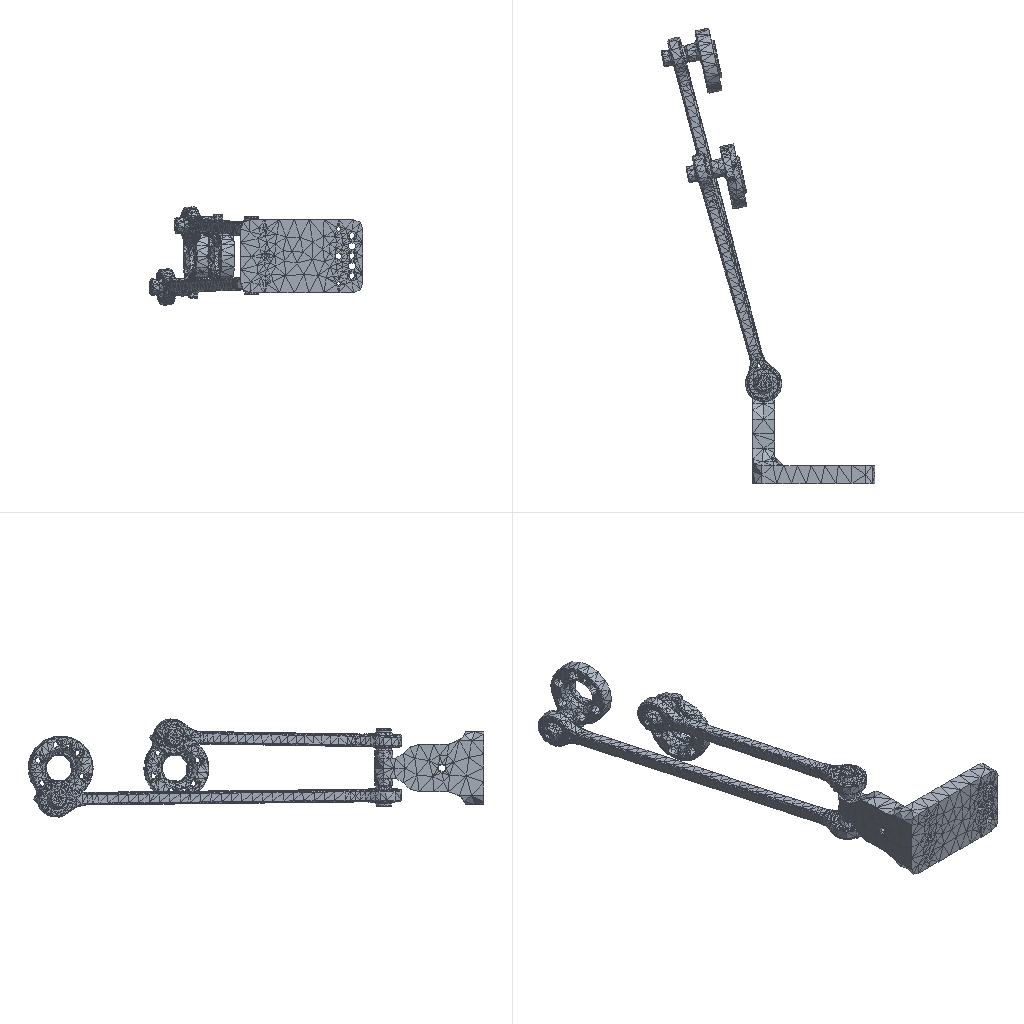Simulation study | ansys workbench
Set-up summary:
category,name,step,type,value,unit,region
solver,ansys_workbench
units,mm-N-s-tonne (MPa),,stated,"/units,MPA"
analysis,LS1,,static
load_step,LS1,LS1,static,nsubst=1; time=1
mesh,nodes,,,43190
mesh,elements,,,31135
element_type,SOLID187,,,21607
element_type,CONTA174,,,5036
element_type,TARGE170,,,4234
element_type,SURF154,,,258
material,Structural Steel,,E,200000,tonne s^-2 mm^-1
material,Structural Steel,,nu,0.3
material,Structural Steel,,density,7.85e-09,tonne mm^-3
material,Structural Steel,,conductivity,60.5,tonne mm s^-3 C^-1
material,Structural Steel,,specific_heat,4.34e+08,mm^2 s^-2 C^-1
material,Structural Steel,,cte,1.2e-05,C^-1
material,Structural Steel,,permeability,10000
material,Structural Steel,,resistivity,0.00017,ohm mm
load,Define Force Using Surface Effect Elements,LS1,surface-effect pres face 2,0.1,,SURF154 #100
bc,Fixed Supports,model,fixed,[dofs=ALL],,_FIXEDSU
bc,,LS1,fixed,"[dofs=ROTX,ROTY,ROTZ,UX,UZ n=5]",,node list
contact,1,,bonded (always),element=CONTA174
contact,Contact Region 2,,bonded (always),element=CONTA174
contact,Contact Region 3,,bonded (always),element=CONTA174
contact,Contact Region 5,,bonded (always),element=CONTA174
contact,Contact Region 6,,bonded (always),element=CONTA174
contact,Contact Region 8,,bonded (always),element=CONTA174
contact,Contact Region 9,,bonded (always),element=CONTA174
contact,Contact Region 10,,bonded (always),element=CONTA174
contact,Contact Region 11,,bonded (always),element=CONTA174
contact,Contact Region 12,,bonded (always),element=CONTA174
contact,Contact Region 13,,bonded (always),element=CONTA174
contact,Contact Region 15,,bonded (always),element=CONTA174
contact,Contact Region 17,,bonded (always),element=CONTA174
contact,Contact Region 18,,bonded (always),element=CONTA174
contact,Contact Region 19,,bonded (always),element=CONTA174
contact,Contact Region 21,,bonded (always),element=CONTA174
contact,Contact Region 23,,bonded (always),element=CONTA174
contact,Contact Region 24,,bonded (always),element=CONTA174
contact,Contact Region 25,,bonded (always),element=CONTA174
contact,? - ? To ?,,bonded (always),element=CONTA174
contact,? - ? To ?,,bonded (always),element=CONTA174
contact,Contact Region 22,,bonded (always),element=CONTA174
contact,Contact Region 26,,bonded (always),element=CONTA174
contact,Contact Region 27,,bonded (always),element=CONTA174
contact,Contact Region 28,,bonded (always),element=CONTA174
contact,Contact Region 29,,bonded (always),element=CONTA174
contact,Contact Region 30,,bonded (always),element=CONTA174
contact,? - ? To ?,,bonded (always),element=CONTA174
contact,? - ? To ?,,bonded (always),element=CONTA174
contact,contact 30,,bonded (always),element=CONTA174
contact,contact 31,,bonded (always),element=CONTA174
contact,contact 32,,bonded (always),element=CONTA174
contact,contact 33,,bonded (always),element=CONTA174
contact,contact 34,,bonded (always),element=CONTA174
contact,contact 35,,bonded (always),element=CONTA174
contact,contact 36,,bonded (always),element=CONTA174
contact,contact 37,,bonded (always),element=CONTA174
contact,contact 38,,bonded (always),element=CONTA174
named_set,_FIXEDSU,,node,746
named_set,REMOTEDISPALL,,node,1
Ansys APDL input file, long lists of numbers shortened:
/batch
/config,noeldb,1     ! force off writing results to database
*get,_wallstrt,active,,time,wall
! ANSYS input file written by Workbench version 2024 R2
! File used for geometry attach:
/title,wbnew--____ (A5)
! ****** Begin Custom Load Command Snippet ******
/COM, ACT Extensions:
/COM,     LSDYNA, 2024.2
/COM,/COM,     ANSYSMotion, 2024.2
/COM,
! ****** End   Custom Load Command Snippet ******
*DIM,_wb_ProjectScratch_dir,string,248
_wb_ProjectScratch_dir(1) = ''
*DIM,_wb_SolverFiles_dir,string,248
_wb_SolverFiles_dir(1) = ''
*DIM,_wb_userfiles_dir,string,248
_wb_userfiles_dir(1) = ''
/com,--- Data in consistent NMM units. See Solving Units in the help system for more information.
/units,MPA
/nopr
/wb,file,start              !  signify a WB generated input file
/prep7
! Turn off shape checking because checks already performed inside WB mesher.
! See help system for more information.
SHPP,OFF,,NOWARN
/nolist
etcon,set             ! allow ANSYS to choose best KEYOP's for 180x elements, resets any applicable keyopt to MAPDL defaults
/com,*********** Nodes for the whole assembly ***********
nblock,3,,47499
(1i9,3e20.9e3)
        1    -2.462083880E+01     5.415586931E+01     1.953544541E+01
! (43180 more lines like these left out)
-1
/com,*********** Nodes for all Remote Points ***********
nblock,3
(1i9,3e20.9e3)
    43192    -1.163425513E+00    -1.361181627E-06     3.324158420E-02
! (8 more lines like these left out)
-1
/wb,elem,start            !  set before creation of elements
/com,*********** Elements for Body 1 'BNN51-GEG6C_ASM|BNN51-GEG6C-1|BNN51-GEG6C-1' ***********
et,1,187
eblock,19,solid,,195
(19i9)
        1        1        1        1        0        0        0        0       10        0        1       27       76       84       77      250      436      252      251
! (389 more lines like these left out)
-1
/com,*********** Elements for Body 2 'BNN51-GEG6C_ASM|BNN51-GEG6C-2|BNN51-GEG6C-2' ***********
et,2,187
eblock,19,solid,,134
(19i9)
        2        2        2        2        0        0        0        0       10        0      196      455      508      507      495      609      787      608      607
! (267 more lines like these left out)
-1
/com,*********** Elements for Body 3 'BNN51-GEG6C5097213_ASM|BNN51-GEG6C-2|BNN51-GEG6C-2' ***********
et,3,187
eblock,19,solid,,134
(19i9)
        3        3        3        3        0        0        0        0       10        0      330      805      858      857      845      959     1137      958      957
! (267 more lines like these left out)
-1
/com,*********** Elements for Body 4 'BNN51-GEG6C5097213_ASM|BNN51-GEG6C-1|BNN51-GEG6C-1' ***********
et,4,187
eblock,19,solid,,195
(19i9)
        4        4        4        4        0        0        0        0       10        0      464     1172     1221     1229     1222     1395     1581     1397     1396
! (389 more lines like these left out)
-1
/com,*********** Elements for Body 5 'GHA-0000182_ASM|BNN51-GEG6C6483096_ASM|BNN51-GEG6C-1|BNN51-GEG6C-1' ***********
et,5,187
eblock,19,solid,,195
(19i9)
        5        5        5        5        0        0        0        0       10        0      659     1617     1666     1674     1667     1840     2026     1842     1841
! (389 more lines like these left out)
-1
/com,*********** Elements for Body 6 'GHA-0000182_ASM|BNN51-GEG6C6483096_ASM|BNN51-GEG6C-2|BNN51-GEG6C-2' ***********
et,6,187
eblock,19,solid,,134
(19i9)
        6        6        6        6        0        0        0        0       10        0      854     2045     2098     2097     2085     2199     2377     2198     2197
! (267 more lines like these left out)
-1
/com,*********** Elements for Body 7 'GHA-0000182_ASM|BNN51-GEG6C5308104_ASM|BNN51-GEG6C-2|BNN51-GEG6C-2' ***********
et,7,187
eblock,19,solid,,134
(19i9)
        7        7        7        7        0        0        0        0       10        0      988     2395     2448     2447     2435     2549     2727     2548     2547
! (267 more lines like these left out)
-1
/com,*********** Elements for Body 8 'GHA-0000182_ASM|BNN51-GEG6C5308104_ASM|BNN51-GEG6C-1|BNN51-GEG6C-1' ***********
et,8,187
eblock,19,solid,,195
(19i9)
        8        8        8        8        0        0        0        0       10        0     1122     2762     2811     2819     2812     2985     3171     2987     2986
! (389 more lines like these left out)
-1
/com,*********** Elements for Body 9 'GHA-0000182_ASM|CBSTSR3-5|CBSTSR3-5' ***********
et,9,187
eblock,19,solid,,829
(19i9)
        9        9        9        9        0        0        0        0       10        0     1317     3260     3454     3349     3449     3982     4492     3976     3981
! (1657 more lines like these left out)
-1
/com,*********** Elements for Body 10 'GHA-0000182_ASM|GHX-0001280|GHX-0001280' ***********
et,10,187
eblock,19,solid,,3467
(19i9)
       10       10       10       10        0        0        0        0       10        0     2146     5277     6021     5785     5417     9449    11413     9445     9439
! (6933 more lines like these left out)
-1
/com,*********** Elements for Body 11 'GHA-0000182_ASM|E-MSB6-15|E-MSB6-15' ***********
et,11,187
eblock,19,solid,,480
(19i9)
       11       11       11       11        0        0        0        0       10        0     5613    12002    12097    12144    12006    12346    12814    12348    12343
! (959 more lines like these left out)
-1
/com,*********** Elements for Body 12 'GHA-0000182_ASM|GHX-0001424|GHX-0001424' ***********
et,12,187
eblock,19,solid,,2733
(19i9)
       12       12       12       12        0        0        0        0       10        0     6093    13364    13827    13762    13741    16638    18195    16636    16635
! (5465 more lines like these left out)
-1
/com,*********** Elements for Body 13 'CBSTSR3-5|CBSTSR3-5' ***********
et,13,187
eblock,19,solid,,829
(19i9)
       13       13       13       13        0        0        0        0       10        0     8826    18337    18531    18426    18526    19059    19569    19053    19058
! (1657 more lines like these left out)
-1
/com,*********** Elements for Body 14 'GHX-0001424|GHX-0001424' ***********
et,14,187
eblock,19,solid,,2733
(19i9)
       14       14       14       14        0        0        0        0       10        0     9655    20291    20754    20689    20668    23565    25122    23563    23562
! (5465 more lines like these left out)
-1
/com,*********** Elements for Body 15 'E-MSB6-15|E-MSB6-15' ***********
et,15,187
eblock,19,solid,,480
(19i9)
       15       15       15       15        0        0        0        0       10        0    12388    25214    25309    25356    25218    25558    26026    25560    25555
! (959 more lines like these left out)
-1
/com,*********** Elements for Body 16 'GHX-0001278|GHX-0001278' ***********
et,16,187
eblock,19,solid,,3367
(19i9)
       16       16       16       16        0        0        0        0       10        0    12868    26645    27335    27190    27308    30628    32646    30625    30627
! (6733 more lines like these left out)
-1
/com,*********** Elements for Body 17 'CBSA4-8|CBSA4-8' ***********
et,17,187
eblock,19,solid,,717
(19i9)
       17       17       17       17        0        0        0        0       10        0    16235    33148    33261    33168    33244    33983    34077    33980    33981
! (1433 more lines like these left out)
-1
/com,*********** Elements for Body 18 'GHX-0001427|GHX-0001427' ***********
et,18,187
eblock,19,solid,,1087
(19i9)
       18       18       18       18        0        0        0        0       10        0    16952    34495    34729    34690    34720    35557    36461    35555    35556
! (2173 more lines like these left out)
-1
/com,*********** Elements for Body 19 'GHX-0001273|GHX-0001273' ***********
et,19,187
eblock,19,solid,,3569
(19i9)
       19       19       19       19        0        0        0        0       10        0    18039    37387    37476    37593    37591    42612    42983    42616    42615
! (7137 more lines like these left out)
-1
/wb,elem,end               !  done creating elements
/com,*********** Send User Defined Coordinate System(s) ***********
local,12,0,-27.5,54.999,17.281,0.,0.,0.
local,13,0,-27.5,55.,-12.719,0.,0.,0.
local,14,0,-58.762,171.736,16.965,0.,0.,0.
local,15,0,-76.802,234.455,-16.924,0.,0.,0.
csys,0
toffst,273.15,      ! Temperature offset from absolute zero
/com,*********** Set Reference Temperature ***********
tref,22.
/wb,mat,start              !  starting to send materials
/com,*********** Send Materials ***********
Temperature = 'TEMP' ! Temperature
MP,DENS,1,7.85e-09,	! tonne mm^-3
MP,ALPX,1,1.2e-05,	! C^-1
MP,C,1,434000000,	! mm^2 s^-2 C^-1
MP,KXX,1,60.5,	! tonne mm s^-3 C^-1
MP,RSVX,1,0.00017,	! ohm mm
MP,EX,1,200000,	! tonne s^-2 mm^-1
MP,NUXY,1,0.3,
MP,MURX,1,10000,
Temperature = 'TEMP' ! Temperature
MP,DENS,2,7.85e-09,	! tonne mm^-3
MP,ALPX,2,1.2e-05,	! C^-1
MP,C,2,434000000,	! mm^2 s^-2 C^-1
MP,KXX,2,60.5,	! tonne mm s^-3 C^-1
MP,RSVX,2,0.00017,	! ohm mm
MP,EX,2,200000,	! tonne s^-2 mm^-1
MP,NUXY,2,0.3,
MP,MURX,2,10000,
Temperature = 'TEMP' ! Temperature
MP,DENS,3,7.85e-09,	! tonne mm^-3
MP,ALPX,3,1.2e-05,	! C^-1
MP,C,3,434000000,	! mm^2 s^-2 C^-1
MP,KXX,3,60.5,	! tonne mm s^-3 C^-1
MP,RSVX,3,0.00017,	! ohm mm
MP,EX,3,200000,	! tonne s^-2 mm^-1
MP,NUXY,3,0.3,
MP,MURX,3,10000,
Temperature = 'TEMP' ! Temperature
MP,DENS,4,7.85e-09,	! tonne mm^-3
MP,ALPX,4,1.2e-05,	! C^-1
MP,C,4,434000000,	! mm^2 s^-2 C^-1
MP,KXX,4,60.5,	! tonne mm s^-3 C^-1
MP,RSVX,4,0.00017,	! ohm mm
MP,EX,4,200000,	! tonne s^-2 mm^-1
MP,NUXY,4,0.3,
MP,MURX,4,10000,
Temperature = 'TEMP' ! Temperature
MP,DENS,5,7.85e-09,	! tonne mm^-3
MP,ALPX,5,1.2e-05,	! C^-1
MP,C,5,434000000,	! mm^2 s^-2 C^-1
MP,KXX,5,60.5,	! tonne mm s^-3 C^-1
MP,RSVX,5,0.00017,	! ohm mm
MP,EX,5,200000,	! tonne s^-2 mm^-1
MP,NUXY,5,0.3,
MP,MURX,5,10000,
Temperature = 'TEMP' ! Temperature
MP,DENS,6,7.85e-09,	! tonne mm^-3
MP,ALPX,6,1.2e-05,	! C^-1
MP,C,6,434000000,	! mm^2 s^-2 C^-1
MP,KXX,6,60.5,	! tonne mm s^-3 C^-1
MP,RSVX,6,0.00017,	! ohm mm
MP,EX,6,200000,	! tonne s^-2 mm^-1
MP,NUXY,6,0.3,
MP,MURX,6,10000,
Temperature = 'TEMP' ! Temperature
MP,DENS,7,7.85e-09,	! tonne mm^-3
MP,ALPX,7,1.2e-05,	! C^-1
MP,C,7,434000000,	! mm^2 s^-2 C^-1
MP,KXX,7,60.5,	! tonne mm s^-3 C^-1
MP,RSVX,7,0.00017,	! ohm mm
MP,EX,7,200000,	! tonne s^-2 mm^-1
MP,NUXY,7,0.3,
MP,MURX,7,10000,
Temperature = 'TEMP' ! Temperature
MP,DENS,8,7.85e-09,	! tonne mm^-3
MP,ALPX,8,1.2e-05,	! C^-1
MP,C,8,434000000,	! mm^2 s^-2 C^-1
MP,KXX,8,60.5,	! tonne mm s^-3 C^-1
MP,RSVX,8,0.00017,	! ohm mm
MP,EX,8,200000,	! tonne s^-2 mm^-1
MP,NUXY,8,0.3,
MP,MURX,8,10000,
Temperature = 'TEMP' ! Temperature
MP,DENS,9,7.85e-09,	! tonne mm^-3
MP,ALPX,9,1.2e-05,	! C^-1
MP,C,9,434000000,	! mm^2 s^-2 C^-1
MP,KXX,9,60.5,	! tonne mm s^-3 C^-1
MP,RSVX,9,0.00017,	! ohm mm
MP,EX,9,200000,	! tonne s^-2 mm^-1
! (92 more lines like these left out)
/wb,mat,end                !  done sending materials
!************************* Model Summary ********************
!BNN51-GEG6C_ASM|BNN51-GEG6C-1|BNN51-GEG6C-1,	ç»æé¢,	matid,	1
!BNN51-GEG6C_ASM|BNN51-GEG6C-2|BNN51-GEG6C-2,	ç»æé¢,	matid,	2
!BNN51-GEG6C5097213_ASM|BNN51-GEG6C-2|BNN51-GEG6C-2,	ç»æé¢,	matid,	3
!BNN51-GEG6C5097213_ASM|BNN51-GEG6C-1|BNN51-GEG6C-1,	ç»æé¢,	matid,	4
!GHA-0000182_ASM|BNN51-GEG6C6483096_ASM|BNN51-GEG6C-1|BNN51-GEG6C-1,	ç»æé¢,	matid,	5
!GHA-0000182_ASM|BNN51-GEG6C6483096_ASM|BNN51-GEG6C-2|BNN51-GEG6C-2,	ç»æé¢,	matid,	6
!GHA-0000182_ASM|BNN51-GEG6C5308104_ASM|BNN51-GEG6C-2|BNN51-GEG6C-2,	ç»æé¢,	matid,	7
!GHA-0000182_ASM|BNN51-GEG6C5308104_ASM|BNN51-GEG6C-1|BNN51-GEG6C-1,	ç»æé¢,	matid,	8
!GHA-0000182_ASM|CBSTSR3-5|CBSTSR3-5,	ç»æé¢,	matid,	9
!GHA-0000182_ASM|GHX-0001280|GHX-0001280,	ç»æé¢,	matid,	10
!GHA-0000182_ASM|E-MSB6-15|E-MSB6-15,	ç»æé¢,	matid,	11
!GHA-0000182_ASM|GHX-0001424|GHX-0001424,	ç»æé¢,	matid,	12
!CBSTSR3-5|CBSTSR3-5,	ç»æé¢,	matid,	13
!GHX-0001424|GHX-0001424,	ç»æé¢,	matid,	14
!E-MSB6-15|E-MSB6-15,	ç»æé¢,	matid,	15
!GHX-0001278|GHX-0001278,	ç»æé¢,	matid,	16
!CBSA4-8|CBSA4-8,	ç»æé¢,	matid,	17
!GHX-0001427|GHX-0001427,	ç»æé¢,	matid,	18
!GHX-0001273|GHX-0001273,	ç»æé¢,	matid,	19
!************************* End Model Summary ********************
! get the diagonal of the bounding box. Needed later for other things
*get,_xmin,node,,mnloc,x
*get,_ymin,node,,mnloc,y
*get,_zmin,node,,mnloc,z
*get,_xmax,node,,mxloc,x
*get,_ymax,node,,mxloc,y
*get,_zmax,node,,mxloc,z
_ASMDIAG=(_xmax-_xmin)*(_xmax-_xmin)+(_ymax-_ymin)*(_ymax-_ymin)+(_zmax-_zmin)*(_zmax-_zmin)
_ASMDIAG=SQRT(_ASMDIAG)
/wb,contact,start          !  starting to send contact
/com,*********** Create Contact "1" ***********
/com,            Real Constant Set For Above Contact Is 21 & 20
*set,tid,21
*set,cid,20
r,tid
r,cid
et,tid,170
et,cid,174
eblock,10,,,84
(15i9)
    34886       21       21       21        0       21       22       74       74      217      224       74      220
! (83 more lines like these left out)
-1
eblock,10,,,84
(15i9)
    34970       20       20       20        0       21       22       74       74      217      224       74      220
! (83 more lines like these left out)
-1
eblock,10,,,52
(15i9)
    35054       20       21       20        0      447      459      472      472      530      640      472      532
! (51 more lines like these left out)
-1
eblock,10,,,52
(15i9)
    35106       21       20       21        0      447      459      472      472      530      640      472      532
! (51 more lines like these left out)
-1
keyo,cid,8,2               ! auto create asymmetric contact (from Program Controlled setting)
keyo,cid,10,0              ! adjust contact stiffness each NR iteration (from Program Controlled setting)
keyo,cid,12,5              ! bonded always
keyo,cid,18,1              ! small sliding turned on by application
keyo,cid,2,2               ! MPC for bonded contacts (from Program Controlled setting)
keyo,tid,5,0               ! Automatic constraint type detection
keyo,cid,4,2               ! on nodal point - normal to target surface (from Program Controlled setting)
keyo,cid,9,1               ! ignore initial gaps/penetration
keyo,cid,7,0               ! No Prediction
rmod,tid,3,10.      ! FKN
rmod,tid,5,0.       ! ICONT
rmod,tid,6,0.       ! PINB
rmod,tid,10,0.      ! CNOF
rmod,tid,12,0.      ! FKT
rmod,tid,36,80      ! WB DSID
rmod,cid,3,10.      ! FKN
rmod,cid,5,0.       ! ICONT
rmod,cid,6,0.       ! PINB
rmod,cid,10,0.      ! CNOF
rmod,cid,12,0.      ! FKT
rmod,cid,36,80      ! WB DSID
/com,*********** Create Contact "½Ó´¥ÇøÓò 2" ***********
/com,            Real Constant Set For Above Contact Is 23 & 22
*set,tid,23
*set,cid,22
r,tid
r,cid
et,tid,170
et,cid,174
eblock,10,,,60
(15i9)
    35158       23       23       23        0       61       60       78       78      401      402       78      405
! (59 more lines like these left out)
-1
eblock,10,,,60
(15i9)
    35218       22       22       22        0       61       60       78       78      401      402       78      405
! (59 more lines like these left out)
-1
eblock,10,,,116
(15i9)
    35278       22       23       22        0    34601    34415    34593    34593    35051    35050    34593    36059
! (115 more lines like these left out)
-1
eblock,10,,,116
(15i9)
    35394       23       22       23        0    34601    34415    34593    34593    35051    35050    34593    36059
! (115 more lines like these left out)
-1
keyo,cid,8,2               ! auto create asymmetric contact (from Program Controlled setting)
keyo,cid,10,0              ! adjust contact stiffness each NR iteration (from Program Controlled setting)
keyo,cid,12,5              ! bonded always
keyo,cid,18,1              ! small sliding turned on by application
keyo,cid,2,2               ! MPC for bonded contacts (from Program Controlled setting)
keyo,tid,5,0               ! Automatic constraint type detection
keyo,cid,4,2               ! on nodal point - normal to target surface (from Program Controlled setting)
keyo,cid,9,1               ! ignore initial gaps/penetration
keyo,cid,7,0               ! No Prediction
rmod,tid,3,10.      ! FKN
rmod,tid,5,0.       ! ICONT
rmod,tid,6,0.       ! PINB
rmod,tid,10,0.      ! CNOF
rmod,tid,12,0.      ! FKT
rmod,tid,36,83      ! WB DSID
rmod,cid,3,10.      ! FKN
rmod,cid,5,0.       ! ICONT
rmod,cid,6,0.       ! PINB
rmod,cid,10,0.      ! CNOF
rmod,cid,12,0.      ! FKT
rmod,cid,36,83      ! WB DSID
/com,*********** Create Contact "½Ó´¥ÇøÓò 3" ***********
/com,            Real Constant Set For Above Contact Is 25 & 24
*set,tid,25
*set,cid,24
r,tid
r,cid
et,tid,170
et,cid,174
eblock,10,,,20
(15i9)
    35510       25       25       25        0       56       61       57       57      384      388       57      382
! (19 more lines like these left out)
-1
eblock,10,,,20
(15i9)
    35530       24       24       24        0       56       61       57       57      384      388       57      382
! (19 more lines like these left out)
-1
eblock,10,,,18
(15i9)
    35550       24       25       24        0    36850    36851    37081    37081    39882    39889    37081    39883
! (17 more lines like these left out)
-1
eblock,10,,,18
(15i9)
    35568       25       24       25        0    36850    36851    37081    37081    39882    39889    37081    39883
! (17 more lines like these left out)
-1
keyo,cid,8,2               ! auto create asymmetric contact (from Program Controlled setting)
keyo,cid,10,0              ! adjust contact stiffness each NR iteration (from Program Controlled setting)
keyo,cid,12,5              ! bonded always
keyo,cid,18,1              ! small sliding turned on by application
keyo,cid,2,2               ! MPC for bonded contacts (from Program Controlled setting)
keyo,tid,5,0               ! Automatic constraint type detection
keyo,cid,4,2               ! on nodal point - normal to target surface (from Program Controlled setting)
keyo,cid,9,1               ! ignore initial gaps/penetration
keyo,cid,7,0               ! No Prediction
rmod,tid,3,10.      ! FKN
rmod,tid,5,0.       ! ICONT
rmod,tid,6,0.       ! PINB
rmod,tid,10,0.      ! CNOF
rmod,tid,12,0.      ! FKT
rmod,tid,36,86      ! WB DSID
rmod,cid,3,10.      ! FKN
rmod,cid,5,0.       ! ICONT
rmod,cid,6,0.       ! PINB
rmod,cid,10,0.      ! CNOF
rmod,cid,12,0.      ! FKT
rmod,cid,36,86      ! WB DSID
/com,*********** Create Contact "½Ó´¥ÇøÓò 5" ***********
/com,            Real Constant Set For Above Contact Is 27 & 26
*set,tid,27
*set,cid,26
r,tid
r,cid
et,tid,170
et,cid,174
eblock,10,,,52
(15i9)
    35586       27       27       27        0      797      809      822      822      880      990      822      882
! (51 more lines like these left out)
-1
eblock,10,,,52
(15i9)
    35638       26       26       26        0      797      809      822      822      880      990      822      882
! (51 more lines like these left out)
-1
eblock,10,,,84
(15i9)
    35690       26       27       26        0     1192     1178     1208     1208     1418     1419     1208     1494
! (83 more lines like these left out)
-1
eblock,10,,,84
(15i9)
    35774       27       26       27        0     1192     1178     1208     1208     1418     1419     1208     1494
! (83 more lines like these left out)
-1
keyo,cid,8,2               ! auto create asymmetric contact (from Program Controlled setting)
keyo,cid,10,0              ! adjust contact stiffness each NR iteration (from Program Controlled setting)
keyo,cid,12,5              ! bonded always
keyo,cid,18,1              ! small sliding turned on by application
keyo,cid,2,2               ! MPC for bonded contacts (from Program Controlled setting)
keyo,tid,5,0               ! Automatic constraint type detection
keyo,cid,4,2               ! on nodal point - normal to target surface (from Program Controlled setting)
keyo,cid,9,1               ! ignore initial gaps/penetration
keyo,cid,7,0               ! No Prediction
rmod,tid,3,10.      ! FKN
rmod,tid,5,0.       ! ICONT
rmod,tid,6,0.       ! PINB
rmod,tid,10,0.      ! CNOF
rmod,tid,12,0.      ! FKT
rmod,tid,36,92      ! WB DSID
rmod,cid,3,10.      ! FKN
rmod,cid,5,0.       ! ICONT
rmod,cid,6,0.       ! PINB
rmod,cid,10,0.      ! CNOF
rmod,cid,12,0.      ! FKT
rmod,cid,36,92      ! WB DSID
/com,*********** Create Contact "½Ó´¥ÇøÓò 6" ***********
/com,            Real Constant Set For Above Contact Is 29 & 28
*set,tid,29
*set,cid,28
r,tid
r,cid
et,tid,170
et,cid,174
eblock,10,,,6
(15i9)
    35858       29       29       29        0      818      863      819      819     1026     1028      819     1024
    35859       29       29       29        0      820      866      821      821     1033     1034      821     1031
    35860       29       29       29        0      819      865      820      820     1030     1032      820     1027
    35861       29       29       29        0      820      865      866      866     1032     1144      866     1033
    35862       29       29       29        0      819      864      865      865     1029     1143      865     1030
    35863       29       29       29        0      819      863      864      864     1028     1142      864     1029
-1
eblock,10,,,6
(15i9)
    35864       28       28       28        0      818      863      819      819     1026     1028      819     1024
    35865       28       28       28        0      820      866      821      821     1033     1034      821     1031
    35866       28       28       28        0      819      865      820      820     1030     1032      820     1027
    35867       28       28       28        0      820      865      866      866     1032     1144      866     1033
    35868       28       28       28        0      819      864      865      865     1029     1143      865     1030
    35869       28       28       28        0      819      863      864      864     1028     1142      864     1029
-1
eblock,10,,,37
(15i9)
    35870       28       29       28        0    18303    18304    18480    18480    18895    18898    18480    18896
! (36 more lines like these left out)
-1
eblock,10,,,37
(15i9)
    35907       29       28       29        0    18303    18304    18480    18480    18895    18898    18480    18896
! (36 more lines like these left out)
-1
keyo,cid,8,2               ! auto create asymmetric contact (from Program Controlled setting)
keyo,cid,10,0              ! adjust contact stiffness each NR iteration (from Program Controlled setting)
keyo,cid,12,5              ! bonded always
keyo,cid,18,1              ! small sliding turned on by application
keyo,cid,2,2               ! MPC for bonded contacts (from Program Controlled setting)
keyo,tid,5,0               ! Automatic constraint type detection
keyo,cid,4,2               ! on nodal point - normal to target surface (from Program Controlled setting)
keyo,cid,9,1               ! ignore initial gaps/penetration
keyo,cid,7,0               ! No Prediction
rmod,tid,3,10.      ! FKN
rmod,tid,5,0.       ! ICONT
rmod,tid,6,0.       ! PINB
rmod,tid,10,0.      ! CNOF
rmod,tid,12,0.      ! FKT
rmod,tid,36,95      ! WB DSID
rmod,cid,3,10.      ! FKN
rmod,cid,5,0.       ! ICONT
rmod,cid,6,0.       ! PINB
rmod,cid,10,0.      ! CNOF
rmod,cid,12,0.      ! FKT
rmod,cid,36,95      ! WB DSID
! (24 more sections like these left out)
/wb,contact,end            !  done creating contacts
/golist
/wb,load,start             !  starting to send loads
/com,*********** Fixed Supports ***********
CMBLOCK,_FIXEDSU,NODE,      746
(8i10)
     12941     12943     12944     12945     12974     12976     12977     12978
! (93 more lines like these left out)
cmsel,s,_FIXEDSU
d,all,all
nsel,all
/com,*********** Create Remote Point "ÄÚ²¿Ô¶³Ìµã 9" ***********
! -------- Remote Point Used by "Ô¶³ÌÎ»ÒÆ" --------
*set,tid,79
*set,cid,78
et,cid,174
et,tid,170
keyo,tid,2,1               ! Don't fix the pilot node
keyo,tid,4,111111
keyo,cid,12,5              ! Bonded Contact
keyo,cid,4,1               ! Deformable RBE3 style load
keyo,cid,2,2               ! MPC style contact
eblock,10,,,258
(15i9)
    43354       78       78       78        0    37186    37201    37212    37212    41622    41729    37212    41624
! (257 more lines like these left out)
-1
*set,_npilot,43192
_npilot213=_npilot
type,tid
mat ,cid
real,cid
tshape,pilo
en,43612,_npilot
tshape
/com,*********** Create Remote Point "ÄÚ²¿Ô¶³Ìµã 10" ***********
! -------- Remote Point Used by "»Ø×ª - ÎÞÑ¡Ôñ Î»ÓÚ ÎÞÑ¡Ôñ" --------
*set,tid,81
*set,cid,80
et,cid,174
et,tid,170
keyo,tid,2,1               ! Don't fix the pilot node
keyo,tid,4,111111
keyo,cid,12,5              ! Bonded Contact
keyo,cid,4,2               ! Rigid CERIG style load
keyo,cid,2,2               ! MPC style contact
eblock,10,,,84
(15i9)
    43613       80       80       80        0       21       22       74       74      217      224       74      220
! (83 more lines like these left out)
-1
*set,_npilot,43193
_npilot277=_npilot
type,tid
mat ,cid
real,cid
tshape,pilo
en,43697,_npilot
tshape
/com,*********** Create Remote Point "ÄÚ²¿Ô¶³Ìµã 11" ***********
! -------- Remote Point Used by "»Ø×ª - ÎÞÑ¡Ôñ Î»ÓÚ ÎÞÑ¡Ôñ" --------
*set,tid,83
*set,cid,82
et,cid,174
et,tid,170
keyo,tid,2,1               ! Don't fix the pilot node
keyo,tid,4,111111
keyo,cid,12,5              ! Bonded Contact
keyo,cid,4,2               ! Rigid CERIG style load
keyo,cid,2,2               ! MPC style contact
eblock,10,,,52
(15i9)
    43698       82       82       82        0      447      459      472      472      530      640      472      532
! (51 more lines like these left out)
-1
*set,_npilot,43194
_npilot278=_npilot
type,tid
mat ,cid
real,cid
tshape,pilo
en,43750,_npilot
tshape
/com,*********** Create Remote Point "ÄÚ²¿Ô¶³Ìµã 12" ***********
! -------- Remote Point Used by "»Ø×ª - ÎÞÑ¡Ôñ Î»ÓÚ ÎÞÑ¡Ôñ" --------
*set,tid,85
*set,cid,84
et,cid,174
et,tid,170
keyo,tid,2,1               ! Don't fix the pilot node
keyo,tid,4,111111
keyo,cid,12,5              ! Bonded Contact
keyo,cid,4,2               ! Rigid CERIG style load
keyo,cid,2,2               ! MPC style contact
eblock,10,,,84
(15i9)
    43751       84       84       84        0     2756     2757     2809     2809     2952     2959     2809     2955
! (83 more lines like these left out)
-1
*set,_npilot,43195
_npilot285=_npilot
type,tid
mat ,cid
real,cid
tshape,pilo
en,43835,_npilot
tshape
/com,*********** Create Remote Point "ÄÚ²¿Ô¶³Ìµã 13" ***********
! -------- Remote Point Used by "»Ø×ª - ÎÞÑ¡Ôñ Î»ÓÚ ÎÞÑ¡Ôñ" --------
*set,tid,87
*set,cid,86
et,cid,174
et,tid,170
keyo,tid,2,1               ! Don't fix the pilot node
keyo,tid,4,111111
keyo,cid,12,5              ! Bonded Contact
keyo,cid,4,2               ! Rigid CERIG style load
keyo,cid,2,2               ! MPC style contact
eblock,10,,,52
(15i9)
    43836       86       86       86        0     2387     2399     2412     2412     2470     2580     2412     2472
! (51 more lines like these left out)
-1
*set,_npilot,43196
_npilot286=_npilot
type,tid
mat ,cid
real,cid
tshape,pilo
en,43888,_npilot
tshape
! (4 more sections like these left out)
/com,*********** Create Joint "»Ø×ª - ÎÞÑ¡Ôñ Î»ÓÚ ÎÞÑ¡Ôñ" ***********
/com,            Real Constant Set For Above Joint Is 96
! Joint Element Type Declaration and Definition using MPC184
*set,_jid,96
et,_jid,184
keyo,_jid,1,6           ! Revolute Joint
keyo,_jid,4,1           ! Z Axis is revolute axis
sectype,_jid, joint, revo, _wbjoint
secjoint,,12,12
mat,_jid
real,_jid
type,_jid
secnum,_jid
en,34876,43193,43194      ! body to body joint
/com,*********** Create Joint "»Ø×ª - ÎÞÑ¡Ôñ Î»ÓÚ ÎÞÑ¡Ôñ" ***********
/com,            Real Constant Set For Above Joint Is 97
! Joint Element Type Declaration and Definition using MPC184
*set,_jid,97
et,_jid,184
keyo,_jid,1,6           ! Revolute Joint
keyo,_jid,4,1           ! Z Axis is revolute axis
sectype,_jid, joint, revo, _wbjoint
secjoint,,13,13
mat,_jid
real,_jid
type,_jid
secnum,_jid
en,34879,43195,43196      ! body to body joint
/com,*********** Create Joint "»Ø×ª - ÎÞÑ¡Ôñ Î»ÓÚ ÎÞÑ¡Ôñ" ***********
/com,            Real Constant Set For Above Joint Is 98
! Joint Element Type Declaration and Definition using MPC184
*set,_jid,98
et,_jid,184
keyo,_jid,1,6           ! Revolute Joint
keyo,_jid,4,1           ! Z Axis is revolute axis
sectype,_jid, joint, revo, _wbjoint
secjoint,,14,14
mat,_jid
real,_jid
type,_jid
secnum,_jid
en,34882,43197,43198      ! body to body joint
/com,*********** Create Joint "»Ø×ª - ÎÞÑ¡Ôñ Î»ÓÚ ÎÞÑ¡Ôñ" ***********
/com,            Real Constant Set For Above Joint Is 99
! Joint Element Type Declaration and Definition using MPC184
*set,_jid,99
et,_jid,184
keyo,_jid,1,6           ! Revolute Joint
keyo,_jid,4,1           ! Z Axis is revolute axis
sectype,_jid, joint, revo, _wbjoint
secjoint,,15,15
mat,_jid
real,_jid
type,_jid
secnum,_jid
en,34885,43199,43200      ! body to body joint
/com,*********** Define Force Using Surface Effect Elements ***********
local,16,0,0.,0.,0.,0.,0.,0.
csys,0
et,100,154
mat,100
eblock,10,,,258
(15i9)
    44165      100      100      100       16    37186    37201    37212    37212    41622    41729    37212    41624
! (257 more lines like these left out)
-1
esel,s,type,,100
keyop,100,2,1       ! Apply load in local coordinate system
keyop,100,7,1       ! Use original area so load is constant in large deformation
esel,all
/com,*********** Construct Remote Displacement ***********
/COM,*** Create a component for all remote displacements ***
CMBLOCK,REMOTEDISPALL,NODE,        1
(8i10)
     43192
/gst,on,on
fini
*get,_numnode,node,0,count
*get,_numelem,elem,0,count
*get, _MAXELEMNUM, elem, 0, NUM, MAX
*get, _MAXNODENUM, node, 0, NUM, MAX
*get, _MAXELEMTYPE, etyp, 0, NUM, MAX
*get, _MAXREALCONST, rcon, 0, NUM, MAX
/go
/wb,load,end               !  done creating loads
/com,--- Number of total nodes = %_numnode%
/com,--- Number of contact elements = 9528
/com,--- Number of spring elements = 0
/com,--- Number of bearing elements = 0
/com,--- Number of solid elements = 21607
/com,--- Number of condensed parts = 0
/com,--- Number of total elements = %_numelem%
*get,_wallbsol,active,,time,wall
/com,****************************************************************************
/com,*************************    SOLUTION       ********************************
/com,****************************************************************************
/solu
antype,0                   ! static analysis
_thickRatio=0.316   ! Ratio of thick parts in the model
eqsl,sparse,,,,,1
cntr,print,1               ! print out contact info and also make no initial contact an error
dmpoption,emat,no             ! Don't combine emat file for DANSYS
dmpoption,esav,no             ! Don't combine esav file for DANSYS
nldiag,cont,iter           ! print out contact info each equilibrium iteration
rescontrol,,none                 ! Do not keep any restart files
/com,****************************************************
/com,******************* SOLVE FOR LS 1 OF 1 ****************
esel,s,type,,100
nsle
sfe,all,1,pres,1,0.
sfe,all,2,pres,1,9.99998143238564e-002
sfe,all,3,pres,1,0.
nsel,all
esel,all
d,43192,ux,0.
d,43192,uz,0.
d,43192,rotx,0.
d,43192,roty,0.
d,43192,rotz,0.
/nopr
/gopr
nsub,1,1,1
time,1.
outres,erase
outres,all,none
outres,nsol,all,
outres,rsol,all
outres,eangl,all
outres,etmp,all
outres,veng,all
outres,strs,all,
outres,epel,all,
outres,eppl,all,
outres,cont,all,
/nopr
esel,s,type,,96
esel,a,type,,97,99
cm,_elmisc,elem
esel,all
/gopr
outres,misc,all,_elmisc
! *********** WB SOLVE COMMAND ***********
! check interactive state
*get,ANSINTER_,active,,int
*if,ANSINTER_,ne,0,then
/eof
*endif
solve
/com *************** Write FE CONNECTORS *********
CEWRITE,file,ce,,INTE
/com,****************************************************
/com,*************** FINISHED SOLVE FOR LS 1 *************
*get,_wallasol,active,,time,wall
/nopr
*get,_numnode,node,0,count
*get,_numelem,elem,0,count
*get, _MAXELEMNUM, elem, 0, NUM, MAX
*get, _MAXNODENUM, node, 0, NUM, MAX,,,INTERNAL
*get, _MAXELEMTYPE, etyp, 0, NUM, MAX
*get, _MAXREALCONST, rcon, 0, NUM, MAX
*get,_NSOLTHREADS,active,0,ntfs
*get,_NSOLPROCESSES,active,0,npfs
/gopr
/post1
xmlo,ENCODING,ISO-8859-1
xmlo,parm
/xml,parm,xml
fini
/gopr
*get,_walldone,active,,time,wall
_preptime=(_wallbsol-_wallstrt)*3600
_solvtime=(_wallasol-_wallbsol)*3600
_posttime=(_walldone-_wallasol)*3600
_totaltim=(_walldone-_wallstrt)*3600
*get,_dlbratio,active,0,solu,dlbr
*get,_combtime,active,0,solu,comb
*get,_ssmode,active,0,solu,ssmm
*get,_ndofs,active,0,solu,ndof
*get,_sol_end_time,active,0,set,time
*if,_sol_end_time,eq,1.,then
/fclean				!clean distributed files
*endif
/com,--- Total number of nodes = %_numnode%
/com,--- Total number of elements = %_numelem%
/com,--- Element load balance ratio = %_dlbratio%
/com,--- Time to combine distributed files = %_combtime%
/com,--- Sparse memory mode = %_ssmode%
/com,--- Number of DOF = %_ndofs%
/wb,file,end               ! done with WB generated input
Results summary:
result,analyses[0].index,,,1
result,analyses[0].system,,,SYS
result,analyses[0].deck,,,deck.dat
result,analyses[0].solve_status,,,completed
result,analyses[0].analysis_type,,,static
result,analyses[0].physics,,,mechanical
result,analyses[0].unit_system,,,"NMM: mm, ton, N, s, mV, mA, degC"
result,analyses[0].n_sets,,,1
result,analyses[0].load_steps[0].set,set=1,,1
result,analyses[0].load_steps[0].time_or_freq,set=1,,1
result,analyses[0].load_steps[0].max_displacement_magnitude,set=1,,152.768
result,analyses[0].load_steps[0].max_von_mises_nodal,set=1,,58.57
result,analyses[0].load_steps[0].reaction_force_sum_xyz[1],set=1,,-0.002833
result,analyses[0].load_steps[0].reaction_force_sum_xyz[2],set=1,,-250
result,analyses[0].load_steps[0].reaction_force_sum_xyz[3],set=1,,0.001453